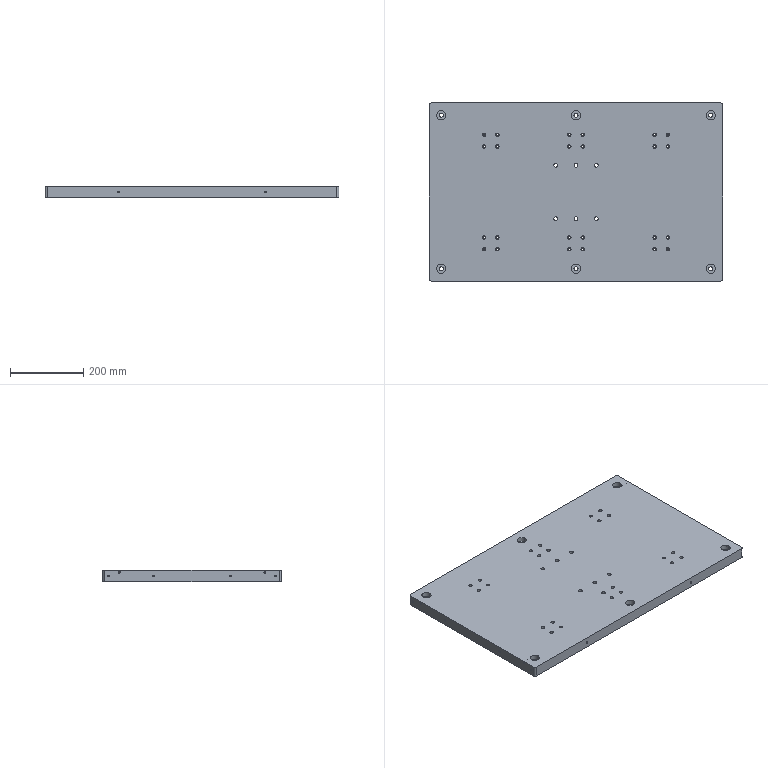NC program | Mastercam | posted with a generic post | part box 800 x 485 x 30 mm
Lines 761 to 1452 of 3510:
( X+CL )
N7560 T20 M6
N7570 G0 G90 G17 G54 X-261.1 Y118. A0. S4000 M3
N7580 G43 H20 Z50. M8
N7590 Z1.2
N7600 G1 Z.2 F600.
N7610 X-259.1 F3000.
N7620 G3 X-257.1 Y120. I0. J2.
N7630 X-265. Y127.9 Z-.05 I-7.9 J0.
N7640 X-272.9 Y120. Z-.3 I0. J-7.9
N7650 X-265. Y112.1 Z-.55 I7.9 J0.
N7660 X-257.1 Y120. Z-.8 I0. J7.9
N7670 X-265. Y127.9 Z-1.05 I-7.9 J0.
N7680 X-272.9 Y120. Z-1.3 I0. J-7.9
N7690 X-265. Y112.1 Z-1.55 I7.9 J0.
N7700 X-257.1 Y120. Z-1.8 I0. J7.9
N7710 X-265. Y127.9 Z-2.05 I-7.9 J0.
N7720 X-272.9 Y120. Z-2.3 I0. J-7.9
N7730 X-265. Y112.1 Z-2.55 I7.9 J0.
N7740 X-257.1 Y120. Z-2.8 I0. J7.9
N7750 X-265. Y127.9 Z-3.05 I-7.9 J0.
N7760 X-272.9 Y120. Z-3.3 I0. J-7.9
N7770 X-265. Y112.1 Z-3.55 I7.9 J0.
N7780 X-257.1 Y120. Z-3.8 I0. J7.9
N7790 X-265. Y127.9 Z-4.05 I-7.9 J0.
N7800 X-272.9 Y120. Z-4.3 I0. J-7.9
N7810 X-265. Y112.1 Z-4.55 I7.9 J0.
N7820 X-257.1 Y120. Z-4.8 I0. J7.9
N7830 X-265. Y127.9 Z-5.05 I-7.9 J0.
N7840 X-272.9 Y120. Z-5.3 I0. J-7.9
N7850 X-265. Y112.1 Z-5.55 I7.9 J0.
N7860 X-257.1 Y120. Z-5.8 I0. J7.9
N7870 X-265. Y127.9 Z-6.05 I-7.9 J0.
N7880 X-272.9 Y120. Z-6.3 I0. J-7.9
N7890 X-265. Y112.1 Z-6.55 I7.9 J0.
N7900 X-257.1 Y120. Z-6.8 I0. J7.9
N7910 X-265. Y127.9 Z-7.05 I-7.9 J0.
N7920 X-272.9 Y120. Z-7.3 I0. J-7.9
N7930 X-265. Y112.1 Z-7.55 I7.9 J0.
N7940 X-257.1 Y120. Z-7.8 I0. J7.9
N7950 X-265. Y127.9 Z-8.05 I-7.9 J0.
N7960 X-272.9 Y120. Z-8.3 I0. J-7.9
N7970 X-265. Y112.1 Z-8.55 I7.9 J0.
N7980 X-257.1 Y120. Z-8.8 I0. J7.9
N7990 X-265. Y127.9 Z-9.05 I-7.9 J0.
N8000 X-272.9 Y120. Z-9.3 I0. J-7.9
N8010 X-265. Y112.1 Z-9.55 I7.9 J0.
N8020 X-257.1 Y120. Z-9.8 I0. J7.9
N8030 X-265. Y127.9 Z-10.05 I-7.9 J0.
N8040 X-272.9 Y120. Z-10.3 I0. J-7.9
N8050 X-265. Y112.1 Z-10.55 I7.9 J0.
N8060 X-257.1 Y120. Z-10.8 I0. J7.9
N8070 X-265. Y127.9 Z-11.05 I-7.9 J0.
N8080 X-272.9 Y120. Z-11.3 I0. J-7.9
N8090 X-265. Y112.1 Z-11.55 I7.9 J0.
N8100 X-257.1 Y120. Z-11.8 I0. J7.9
N8110 X-265. Y127.9 Z-12.05 I-7.9 J0.
N8120 X-272.9 Y120. Z-12.3 I0. J-7.9
N8130 X-265. Y112.1 Z-12.55 I7.9 J0.
N8140 X-257.1 Y120. Z-12.8 I0. J7.9
N8150 X-265. Y127.9 Z-13.05 I-7.9 J0.
N8160 X-272.9 Y120. Z-13.3 I0. J-7.9
N8170 X-265. Y112.1 Z-13.55 I7.9 J0.
N8180 X-257.1 Y120. Z-13.8 I0. J7.9
N8190 X-265. Y127.9 Z-14.05 I-7.9 J0.
N8200 X-272.9 Y120. Z-14.3 I0. J-7.9
N8210 X-265. Y112.1 Z-14.55 I7.9 J0.
N8220 X-257.1 Y120. Z-14.8 I0. J7.9
N8230 X-265. Y127.9 Z-15.05 I-7.9 J0.
N8240 X-272.9 Y120. Z-15.3 I0. J-7.9
N8250 X-265. Y112.1 Z-15.55 I7.9 J0.
N8260 X-257.1 Y120. Z-15.8 I0. J7.9
N8270 X-265. Y127.9 Z-16.05 I-7.9 J0.
N8280 X-272.9 Y120. Z-16.3 I0. J-7.9
N8290 X-265. Y112.1 Z-16.55 I7.9 J0.
N8300 X-257.1 Y120. Z-16.8 I0. J7.9
N8310 X-265. Y127.9 Z-17.05 I-7.9 J0.
N8320 X-272.9 Y120. Z-17.3 I0. J-7.9
N8330 X-265. Y112.1 Z-17.55 I7.9 J0.
N8340 X-257.1 Y120. Z-17.8 I0. J7.9
N8350 X-265. Y127.9 Z-18.05 I-7.9 J0.
N8360 X-272.9 Y120. Z-18.3 I0. J-7.9
N8370 X-265. Y112.1 Z-18.55 I7.9 J0.
N8380 X-257.1 Y120. Z-18.8 I0. J7.9
N8390 X-265. Y127.9 Z-19.05 I-7.9 J0.
N8400 X-272.9 Y120. Z-19.3 I0. J-7.9
N8410 X-265. Y112.1 Z-19.55 I7.9 J0.
N8420 X-257.1 Y120. Z-19.8 I0. J7.9
N8430 X-265. Y127.9 Z-20.05 I-7.9 J0.
N8440 X-272.9 Y120. Z-20.3 I0. J-7.9
N8450 X-265. Y112.1 Z-20.55 I7.9 J0.
N8460 X-257.1 Y120. Z-20.8 I0. J7.9
N8470 X-265. Y127.9 Z-21.05 I-7.9 J0.
N8480 X-272.9 Y120. Z-21.3 I0. J-7.9
N8490 X-265. Y112.1 Z-21.55 I7.9 J0.
N8500 X-257.1 Y120. Z-21.8 I0. J7.9
N8510 X-265. Y127.9 Z-22.05 I-7.9 J0.
N8520 X-272.9 Y120. Z-22.3 I0. J-7.9
N8530 X-265. Y112.1 Z-22.55 I7.9 J0.
N8540 X-257.1 Y120. Z-22.8 I0. J7.9
N8550 X-265. Y127.9 Z-23.05 I-7.9 J0.
N8560 X-272.9 Y120. Z-23.3 I0. J-7.9
N8570 X-265. Y112.1 Z-23.55 I7.9 J0.
N8580 X-257.1 Y120. Z-23.8 I0. J7.9
N8590 X-265. Y127.9 Z-24.05 I-7.9 J0.
N8600 X-272.9 Y120. Z-24.3 I0. J-7.9
N8610 X-265. Y112.1 Z-24.55 I7.9 J0.
N8620 X-257.1 Y120. Z-24.8 I0. J7.9
N8630 X-260.356 Y126.391 Z-24.95 I-7.9 J0.
N8640 X-265. Y127.9 I-4.644 J-6.391
N8650 X-272.9 Y120. I0. J-7.9
N8660 X-265. Y112.1 I7.9 J0.
N8670 X-257.1 Y120. I0. J7.9
N8680 X-260.356 Y126.391 I-7.9 J0.
N8690 X-261.532 Y126.773 I-1.176 J-1.618
N8700 X-263.15 Y125.949 I0. J-2.
N8710 G1 X-264.326 Y124.331
N8720 G0 Z50.
N8730 X-251.1 Y118.
N8740 Z1.2
N8750 G1 Z.2 F600.
N8760 X-249.1 F3000.
N8770 G3 X-247.1 Y120. I0. J2.
N8780 X-265. Y137.9 Z-.05 I-17.9 J0.
N8790 X-282.9 Y120. Z-.3 I0. J-17.9
N8800 X-265. Y102.1 Z-.55 I17.9 J0.
N8810 X-247.1 Y120. Z-.8 I0. J17.9
N8820 X-265. Y137.9 Z-1.05 I-17.9 J0.
N8830 X-282.9 Y120. Z-1.3 I0. J-17.9
N8840 X-265. Y102.1 Z-1.55 I17.9 J0.
N8850 X-247.1 Y120. Z-1.8 I0. J17.9
N8860 X-265. Y137.9 Z-2.05 I-17.9 J0.
N8870 X-282.9 Y120. Z-2.3 I0. J-17.9
N8880 X-265. Y102.1 Z-2.55 I17.9 J0.
N8890 X-247.1 Y120. Z-2.8 I0. J17.9
N8900 X-265. Y137.9 Z-3.05 I-17.9 J0.
N8910 X-282.9 Y120. Z-3.3 I0. J-17.9
N8920 X-265. Y102.1 Z-3.55 I17.9 J0.
N8930 X-247.1 Y120. Z-3.8 I0. J17.9
N8940 X-265. Y137.9 Z-4.05 I-17.9 J0.
N8950 X-282.9 Y120. Z-4.3 I0. J-17.9
N8960 X-265. Y102.1 Z-4.55 I17.9 J0.
N8970 X-247.1 Y120. Z-4.8 I0. J17.9
N8980 X-265. Y137.9 Z-5.05 I-17.9 J0.
N8990 X-282.9 Y120. Z-5.3 I0. J-17.9
N9000 X-265. Y102.1 Z-5.55 I17.9 J0.
N9010 X-247.1 Y120. Z-5.8 I0. J17.9
N9020 X-265. Y137.9 Z-6.05 I-17.9 J0.
N9030 X-282.9 Y120. Z-6.3 I0. J-17.9
N9040 X-265. Y102.1 Z-6.55 I17.9 J0.
N9050 X-247.1 Y120. Z-6.8 I0. J17.9
N9060 X-265. Y137.9 Z-7.05 I-17.9 J0.
N9070 X-282.9 Y120. Z-7.3 I0. J-17.9
N9080 X-265. Y102.1 Z-7.55 I17.9 J0.
N9090 X-247.1 Y120. Z-7.8 I0. J17.9
N9100 X-265. Y137.9 Z-8.05 I-17.9 J0.
N9110 X-282.9 Y120. Z-8.3 I0. J-17.9
N9120 X-265. Y102.1 Z-8.55 I17.9 J0.
N9130 X-247.1 Y120. Z-8.8 I0. J17.9
N9140 X-265. Y137.9 Z-9.05 I-17.9 J0.
N9150 X-282.9 Y120. Z-9.3 I0. J-17.9
N9160 X-265. Y102.1 Z-9.55 I17.9 J0.
N9170 X-247.1 Y120. Z-9.8 I0. J17.9
N9180 X-265. Y137.9 Z-10.05 I-17.9 J0.
N9190 X-282.9 Y120. Z-10.3 I0. J-17.9
N9200 X-265. Y102.1 Z-10.55 I17.9 J0.
N9210 X-247.1 Y120. Z-10.8 I0. J17.9
N9220 X-265. Y137.9 Z-11.05 I-17.9 J0.
N9230 X-282.9 Y120. Z-11.3 I0. J-17.9
N9240 X-265. Y102.1 Z-11.55 I17.9 J0.
N9250 X-247.1 Y120. Z-11.8 I0. J17.9
N9260 X-265. Y137.9 Z-12.05 I-17.9 J0.
N9270 X-282.9 Y120. Z-12.3 I0. J-17.9
N9280 X-265. Y102.1 Z-12.55 I17.9 J0.
N9290 X-247.1 Y120. Z-12.8 I0. J17.9
N9300 X-265. Y137.9 Z-13.05 I-17.9 J0.
N9310 X-282.9 Y120. Z-13.3 I0. J-17.9
N9320 X-265. Y102.1 Z-13.55 I17.9 J0.
N9330 X-247.1 Y120. Z-13.8 I0. J17.9
N9340 X-265. Y137.9 Z-14.05 I-17.9 J0.
N9350 X-282.9 Y120. Z-14.3 I0. J-17.9
N9360 X-265. Y102.1 Z-14.55 I17.9 J0.
N9370 X-247.1 Y120. Z-14.8 I0. J17.9
N9380 X-265. Y137.9 Z-15.05 I-17.9 J0.
N9390 X-282.9 Y120. Z-15.3 I0. J-17.9
N9400 X-265. Y102.1 Z-15.55 I17.9 J0.
N9410 X-247.1 Y120. Z-15.8 I0. J17.9
N9420 X-265. Y137.9 Z-16.05 I-17.9 J0.
N9430 X-282.9 Y120. Z-16.3 I0. J-17.9
N9440 X-265. Y102.1 Z-16.55 I17.9 J0.
N9450 X-247.1 Y120. Z-16.8 I0. J17.9
N9460 X-265. Y137.9 Z-17.05 I-17.9 J0.
N9470 X-282.9 Y120. Z-17.3 I0. J-17.9
N9480 X-265. Y102.1 Z-17.55 I17.9 J0.
N9490 X-247.1 Y120. Z-17.8 I0. J17.9
N9500 X-265. Y137.9 Z-18.05 I-17.9 J0.
N9510 X-282.9 Y120. Z-18.3 I0. J-17.9
N9520 X-265. Y102.1 Z-18.55 I17.9 J0.
N9530 X-247.1 Y120. Z-18.8 I0. J17.9
N9540 X-265. Y137.9 Z-19.05 I-17.9 J0.
N9550 X-282.9 Y120. Z-19.3 I0. J-17.9
N9560 X-265. Y102.1 Z-19.55 I17.9 J0.
N9570 X-247.1 Y120. Z-19.8 I0. J17.9
N9580 X-265. Y137.9 Z-20.05 I-17.9 J0.
N9590 X-282.9 Y120. Z-20.3 I0. J-17.9
N9600 X-265. Y102.1 Z-20.55 I17.9 J0.
N9610 X-247.1 Y120. Z-20.8 I0. J17.9
N9620 X-265. Y137.9 Z-21.05 I-17.9 J0.
N9630 X-282.9 Y120. Z-21.3 I0. J-17.9
N9640 X-265. Y102.1 Z-21.55 I17.9 J0.
N9650 X-247.1 Y120. Z-21.8 I0. J17.9
N9660 X-265. Y137.9 Z-22.05 I-17.9 J0.
N9670 X-282.9 Y120. Z-22.3 I0. J-17.9
N9680 X-265. Y102.1 Z-22.55 I17.9 J0.
N9690 X-247.1 Y120. Z-22.8 I0. J17.9
N9700 X-265. Y137.9 Z-23.05 I-17.9 J0.
N9710 X-282.9 Y120. Z-23.3 I0. J-17.9
N9720 X-265. Y102.1 Z-23.55 I17.9 J0.
N9730 X-247.1 Y120. Z-23.8 I0. J17.9
N9740 X-265. Y137.9 Z-24.05 I-17.9 J0.
N9750 X-282.9 Y120. Z-24.3 I0. J-17.9
N9760 X-265. Y102.1 Z-24.55 I17.9 J0.
N9770 X-247.1 Y120. Z-24.8 I0. J17.9
N9780 X-254.479 Y134.481 Z-24.95 I-17.9 J0.
N9790 X-265. Y137.899 I-10.521 J-14.481
N9800 X-282.899 Y120. I0. J-17.899
N9810 X-265. Y102.101 I17.899 J0.
N9820 X-247.1 Y120. I0. J17.899
N9830 X-254.479 Y134.481 I-17.9 J0.
N9840 X-255.654 Y134.863 I-1.175 J-1.618
N9850 X-257.272 Y134.039 I0. J-2.
N9860 G1 X-258.448 Y132.421
N9870 G0 Z50.
N9880 X3.9 Y118.
N9890 Z1.2
N9900 G1 Z.2 F600.
N9910 X5.9 F3000.
N9920 G3 X7.9 Y120. I0. J2.
N9930 X0. Y127.9 Z-.05 I-7.9 J0.
N9940 X-7.9 Y120. Z-.3 I0. J-7.9
N9950 X0. Y112.1 Z-.55 I7.9 J0.
N9960 X7.9 Y120. Z-.8 I0. J7.9
N9970 X0. Y127.9 Z-1.05 I-7.9 J0.
N9980 X-7.9 Y120. Z-1.3 I0. J-7.9
N9990 X0. Y112.1 Z-1.55 I7.9 J0.
N100 X7.9 Y120. Z-1.8 I0. J7.9
N110 X0. Y127.9 Z-2.05 I-7.9 J0.
N120 X-7.9 Y120. Z-2.3 I0. J-7.9
N130 X0. Y112.1 Z-2.55 I7.9 J0.
N140 X7.9 Y120. Z-2.8 I0. J7.9
N150 X0. Y127.9 Z-3.05 I-7.9 J0.
N160 X-7.9 Y120. Z-3.3 I0. J-7.9
N170 X0. Y112.1 Z-3.55 I7.9 J0.
N180 X7.9 Y120. Z-3.8 I0. J7.9
N190 X0. Y127.9 Z-4.05 I-7.9 J0.
N200 X-7.9 Y120. Z-4.3 I0. J-7.9
N210 X0. Y112.1 Z-4.55 I7.9 J0.
N220 X7.9 Y120. Z-4.8 I0. J7.9
N230 X0. Y127.9 Z-5.05 I-7.9 J0.
N240 X-7.9 Y120. Z-5.3 I0. J-7.9
N250 X0. Y112.1 Z-5.55 I7.9 J0.
N260 X7.9 Y120. Z-5.8 I0. J7.9
N270 X0. Y127.9 Z-6.05 I-7.9 J0.
N280 X-7.9 Y120. Z-6.3 I0. J-7.9
N290 X0. Y112.1 Z-6.55 I7.9 J0.
N300 X7.9 Y120. Z-6.8 I0. J7.9
N310 X0. Y127.9 Z-7.05 I-7.9 J0.
N320 X-7.9 Y120. Z-7.3 I0. J-7.9
N330 X0. Y112.1 Z-7.55 I7.9 J0.
N340 X7.9 Y120. Z-7.8 I0. J7.9
N350 X0. Y127.9 Z-8.05 I-7.9 J0.
N360 X-7.9 Y120. Z-8.3 I0. J-7.9
N370 X0. Y112.1 Z-8.55 I7.9 J0.
N380 X7.9 Y120. Z-8.8 I0. J7.9
N390 X0. Y127.9 Z-9.05 I-7.9 J0.
N400 X-7.9 Y120. Z-9.3 I0. J-7.9
N410 X0. Y112.1 Z-9.55 I7.9 J0.
N420 X7.9 Y120. Z-9.8 I0. J7.9
N430 X0. Y127.9 Z-10.05 I-7.9 J0.
N440 X-7.9 Y120. Z-10.3 I0. J-7.9
N450 X0. Y112.1 Z-10.55 I7.9 J0.
N460 X7.9 Y120. Z-10.8 I0. J7.9
N470 X0. Y127.9 Z-11.05 I-7.9 J0.
N480 X-7.9 Y120. Z-11.3 I0. J-7.9
N490 X0. Y112.1 Z-11.55 I7.9 J0.
N500 X7.9 Y120. Z-11.8 I0. J7.9
N510 X0. Y127.9 Z-12.05 I-7.9 J0.
N520 X-7.9 Y120. Z-12.3 I0. J-7.9
N530 X0. Y112.1 Z-12.55 I7.9 J0.
N540 X7.9 Y120. Z-12.8 I0. J7.9
N550 X0. Y127.9 Z-13.05 I-7.9 J0.
N560 X-7.9 Y120. Z-13.3 I0. J-7.9
N570 X0. Y112.1 Z-13.55 I7.9 J0.
N580 X7.9 Y120. Z-13.8 I0. J7.9
N590 X0. Y127.9 Z-14.05 I-7.9 J0.
N600 X-7.9 Y120. Z-14.3 I0. J-7.9
N610 X0. Y112.1 Z-14.55 I7.9 J0.
N620 X7.9 Y120. Z-14.8 I0. J7.9
N630 X0. Y127.9 Z-15.05 I-7.9 J0.
N640 X-7.9 Y120. Z-15.3 I0. J-7.9
N650 X0. Y112.1 Z-15.55 I7.9 J0.
N660 X7.9 Y120. Z-15.8 I0. J7.9
N670 X0. Y127.9 Z-16.05 I-7.9 J0.
N680 X-7.9 Y120. Z-16.3 I0. J-7.9
N690 X0. Y112.1 Z-16.55 I7.9 J0.
N700 X7.9 Y120. Z-16.8 I0. J7.9
N710 X0. Y127.9 Z-17.05 I-7.9 J0.
N720 X-7.9 Y120. Z-17.3 I0. J-7.9
N730 X0. Y112.1 Z-17.55 I7.9 J0.
N740 X7.9 Y120. Z-17.8 I0. J7.9
N750 X0. Y127.9 Z-18.05 I-7.9 J0.
N760 X-7.9 Y120. Z-18.3 I0. J-7.9
N770 X0. Y112.1 Z-18.55 I7.9 J0.
N780 X7.9 Y120. Z-18.8 I0. J7.9
N790 X0. Y127.9 Z-19.05 I-7.9 J0.
N800 X-7.9 Y120. Z-19.3 I0. J-7.9
N810 X0. Y112.1 Z-19.55 I7.9 J0.
N820 X7.9 Y120. Z-19.8 I0. J7.9
N830 X0. Y127.9 Z-20.05 I-7.9 J0.
N840 X-7.9 Y120. Z-20.3 I0. J-7.9
N850 X0. Y112.1 Z-20.55 I7.9 J0.
N860 X7.9 Y120. Z-20.8 I0. J7.9
N870 X0. Y127.9 Z-21.05 I-7.9 J0.
N880 X-7.9 Y120. Z-21.3 I0. J-7.9
N890 X0. Y112.1 Z-21.55 I7.9 J0.
N900 X7.9 Y120. Z-21.8 I0. J7.9
N910 X0. Y127.9 Z-22.05 I-7.9 J0.
N920 X-7.9 Y120. Z-22.3 I0. J-7.9
N930 X0. Y112.1 Z-22.55 I7.9 J0.
N940 X7.9 Y120. Z-22.8 I0. J7.9
N950 X0. Y127.9 Z-23.05 I-7.9 J0.
N960 X-7.9 Y120. Z-23.3 I0. J-7.9
N970 X0. Y112.1 Z-23.55 I7.9 J0.
N980 X7.9 Y120. Z-23.8 I0. J7.9
N990 X0. Y127.9 Z-24.05 I-7.9 J0.
N1000 X-7.9 Y120. Z-24.3 I0. J-7.9
N1010 X0. Y112.1 Z-24.55 I7.9 J0.
N1020 X7.9 Y120. Z-24.8 I0. J7.9
N1030 X4.644 Y126.391 Z-24.95 I-7.9 J0.
N1040 X0. Y127.9 I-4.644 J-6.391
N1050 X-7.9 Y120. I0. J-7.9
N1060 X0. Y112.1 I7.9 J0.
N1070 X7.9 Y120. I0. J7.9
N1080 X4.644 Y126.391 I-7.9 J0.
N1090 X3.468 Y126.773 I-1.176 J-1.618
N1100 X1.85 Y125.949 I0. J-2.
N1110 G1 X.674 Y124.331
N1120 G0 Z50.
N1130 X13.9 Y118.
N1140 Z1.2
N1150 G1 Z.2 F600.
N1160 X15.9 F3000.
N1170 G3 X17.9 Y120. I0. J2.
N1180 X0. Y137.9 Z-.05 I-17.9 J0.
N1190 X-17.9 Y120. Z-.3 I0. J-17.9
N1200 X0. Y102.1 Z-.55 I17.9 J0.
N1210 X17.9 Y120. Z-.8 I0. J17.9
N1220 X0. Y137.9 Z-1.05 I-17.9 J0.
N1230 X-17.9 Y120. Z-1.3 I0. J-17.9
N1240 X0. Y102.1 Z-1.55 I17.9 J0.
N1250 X17.9 Y120. Z-1.8 I0. J17.9
N1260 X0. Y137.9 Z-2.05 I-17.9 J0.
N1270 X-17.9 Y120. Z-2.3 I0. J-17.9
N1280 X0. Y102.1 Z-2.55 I17.9 J0.
N1290 X17.9 Y120. Z-2.8 I0. J17.9
N1300 X0. Y137.9 Z-3.05 I-17.9 J0.
N1310 X-17.9 Y120. Z-3.3 I0. J-17.9
N1320 X0. Y102.1 Z-3.55 I17.9 J0.
N1330 X17.9 Y120. Z-3.8 I0. J17.9
N1340 X0. Y137.9 Z-4.05 I-17.9 J0.
N1350 X-17.9 Y120. Z-4.3 I0. J-17.9
N1360 X0. Y102.1 Z-4.55 I17.9 J0.
N1370 X17.9 Y120. Z-4.8 I0. J17.9
N1380 X0. Y137.9 Z-5.05 I-17.9 J0.
N1390 X-17.9 Y120. Z-5.3 I0. J-17.9
N1400 X0. Y102.1 Z-5.55 I17.9 J0.
N1410 X17.9 Y120. Z-5.8 I0. J17.9
N1420 X0. Y137.9 Z-6.05 I-17.9 J0.
N1430 X-17.9 Y120. Z-6.3 I0. J-17.9
N1440 X0. Y102.1 Z-6.55 I17.9 J0.
N1450 X17.9 Y120. Z-6.8 I0. J17.9
N1460 X0. Y137.9 Z-7.05 I-17.9 J0.
N1470 X-17.9 Y120. Z-7.3 I0. J-17.9
N1480 X0. Y102.1 Z-7.55 I17.9 J0.
N1490 X17.9 Y120. Z-7.8 I0. J17.9
N1500 X0. Y137.9 Z-8.05 I-17.9 J0.
N1510 X-17.9 Y120. Z-8.3 I0. J-17.9
N1520 X0. Y102.1 Z-8.55 I17.9 J0.
N1530 X17.9 Y120. Z-8.8 I0. J17.9
N1540 X0. Y137.9 Z-9.05 I-17.9 J0.
N1550 X-17.9 Y120. Z-9.3 I0. J-17.9
N1560 X0. Y102.1 Z-9.55 I17.9 J0.
N1570 X17.9 Y120. Z-9.8 I0. J17.9
N1580 X0. Y137.9 Z-10.05 I-17.9 J0.
N1590 X-17.9 Y120. Z-10.3 I0. J-17.9
N1600 X0. Y102.1 Z-10.55 I17.9 J0.
N1610 X17.9 Y120. Z-10.8 I0. J17.9
N1620 X0. Y137.9 Z-11.05 I-17.9 J0.
N1630 X-17.9 Y120. Z-11.3 I0. J-17.9
N1640 X0. Y102.1 Z-11.55 I17.9 J0.
N1650 X17.9 Y120. Z-11.8 I0. J17.9
N1660 X0. Y137.9 Z-12.05 I-17.9 J0.
N1670 X-17.9 Y120. Z-12.3 I0. J-17.9
N1680 X0. Y102.1 Z-12.55 I17.9 J0.
N1690 X17.9 Y120. Z-12.8 I0. J17.9
N1700 X0. Y137.9 Z-13.05 I-17.9 J0.
N1710 X-17.9 Y120. Z-13.3 I0. J-17.9
N1720 X0. Y102.1 Z-13.55 I17.9 J0.
N1730 X17.9 Y120. Z-13.8 I0. J17.9
N1740 X0. Y137.9 Z-14.05 I-17.9 J0.
N1750 X-17.9 Y120. Z-14.3 I0. J-17.9
N1760 X0. Y102.1 Z-14.55 I17.9 J0.
N1770 X17.9 Y120. Z-14.8 I0. J17.9
N1780 X0. Y137.9 Z-15.05 I-17.9 J0.
N1790 X-17.9 Y120. Z-15.3 I0. J-17.9
N1800 X0. Y102.1 Z-15.55 I17.9 J0.
N1810 X17.9 Y120. Z-15.8 I0. J17.9
N1820 X0. Y137.9 Z-16.05 I-17.9 J0.
N1830 X-17.9 Y120. Z-16.3 I0. J-17.9
N1840 X0. Y102.1 Z-16.55 I17.9 J0.
N1850 X17.9 Y120. Z-16.8 I0. J17.9
N1860 X0. Y137.9 Z-17.05 I-17.9 J0.
N1870 X-17.9 Y120. Z-17.3 I0. J-17.9
N1880 X0. Y102.1 Z-17.55 I17.9 J0.
N1890 X17.9 Y120. Z-17.8 I0. J17.9
N1900 X0. Y137.9 Z-18.05 I-17.9 J0.
N1910 X-17.9 Y120. Z-18.3 I0. J-17.9
N1920 X0. Y102.1 Z-18.55 I17.9 J0.
N1930 X17.9 Y120. Z-18.8 I0. J17.9
N1940 X0. Y137.9 Z-19.05 I-17.9 J0.
N1950 X-17.9 Y120. Z-19.3 I0. J-17.9
N1960 X0. Y102.1 Z-19.55 I17.9 J0.
N1970 X17.9 Y120. Z-19.8 I0. J17.9
N1980 X0. Y137.9 Z-20.05 I-17.9 J0.
N1990 X-17.9 Y120. Z-20.3 I0. J-17.9
N2000 X0. Y102.1 Z-20.55 I17.9 J0.
N2010 X17.9 Y120. Z-20.8 I0. J17.9
N2020 X0. Y137.9 Z-21.05 I-17.9 J0.
N2030 X-17.9 Y120. Z-21.3 I0. J-17.9
N2040 X0. Y102.1 Z-21.55 I17.9 J0.
N2050 X17.9 Y120. Z-21.8 I0. J17.9
N2060 X0. Y137.9 Z-22.05 I-17.9 J0.
N2070 X-17.9 Y120. Z-22.3 I0. J-17.9
N2080 X0. Y102.1 Z-22.55 I17.9 J0.
N2090 X17.9 Y120. Z-22.8 I0. J17.9
N2100 X0. Y137.9 Z-23.05 I-17.9 J0.
N2110 X-17.9 Y120. Z-23.3 I0. J-17.9
N2120 X0. Y102.1 Z-23.55 I17.9 J0.
N2130 X17.9 Y120. Z-23.8 I0. J17.9
N2140 X0. Y137.9 Z-24.05 I-17.9 J0.
N2150 X-17.9 Y120. Z-24.3 I0. J-17.9
N2160 X0. Y102.1 Z-24.55 I17.9 J0.
N2170 X17.9 Y120. Z-24.8 I0. J17.9
N2180 X10.521 Y134.481 Z-24.95 I-17.9 J0.
N2190 X0. Y137.899 I-10.521 J-14.481
N2200 X-17.899 Y120. I0. J-17.899
N2210 X0. Y102.101 I17.899 J0.
N2220 X17.9 Y120. I0. J17.899
N2230 X10.521 Y134.481 I-17.9 J0.
N2240 X9.346 Y134.863 I-1.175 J-1.618
N2250 X7.728 Y134.039 I0. J-2.
N2260 G1 X6.552 Y132.421
N2270 G0 Z50.
N2280 X268.9 Y118.
N2290 Z1.2
N2300 G1 Z.2 F600.
N2310 X270.9 F3000.
N2320 G3 X272.9 Y120. I0. J2.
N2330 X265. Y127.9 Z-.05 I-7.9 J0.
N2340 X257.1 Y120. Z-.3 I0. J-7.9
N2350 X265. Y112.1 Z-.55 I7.9 J0.
N2360 X272.9 Y120. Z-.8 I0. J7.9
N2370 X265. Y127.9 Z-1.05 I-7.9 J0.
N2380 X257.1 Y120. Z-1.3 I0. J-7.9
N2390 X265. Y112.1 Z-1.55 I7.9 J0.
N2400 X272.9 Y120. Z-1.8 I0. J7.9
N2410 X265. Y127.9 Z-2.05 I-7.9 J0.
N2420 X257.1 Y120. Z-2.3 I0. J-7.9
N2430 X265. Y112.1 Z-2.55 I7.9 J0.
N2440 X272.9 Y120. Z-2.8 I0. J7.9
N2450 X265. Y127.9 Z-3.05 I-7.9 J0.
N2460 X257.1 Y120. Z-3.3 I0. J-7.9
N2470 X265. Y112.1 Z-3.55 I7.9 J0.
N2480 X272.9 Y120. Z-3.8 I0. J7.9
N2490 X265. Y127.9 Z-4.05 I-7.9 J0.
N2500 X257.1 Y120. Z-4.3 I0. J-7.9
N2510 X265. Y112.1 Z-4.55 I7.9 J0.
N2520 X272.9 Y120. Z-4.8 I0. J7.9
N2530 X265. Y127.9 Z-5.05 I-7.9 J0.
N2540 X257.1 Y120. Z-5.3 I0. J-7.9
N2550 X265. Y112.1 Z-5.55 I7.9 J0.
N2560 X272.9 Y120. Z-5.8 I0. J7.9
N2570 X265. Y127.9 Z-6.05 I-7.9 J0.
N2580 X257.1 Y120. Z-6.3 I0. J-7.9
N2590 X265. Y112.1 Z-6.55 I7.9 J0.
N2600 X272.9 Y120. Z-6.8 I0. J7.9
N2610 X265. Y127.9 Z-7.05 I-7.9 J0.
N2620 X257.1 Y120. Z-7.3 I0. J-7.9
N2630 X265. Y112.1 Z-7.55 I7.9 J0.
N2640 X272.9 Y120. Z-7.8 I0. J7.9
N2650 X265. Y127.9 Z-8.05 I-7.9 J0.
N2660 X257.1 Y120. Z-8.3 I0. J-7.9
N2670 X265. Y112.1 Z-8.55 I7.9 J0.
N2680 X272.9 Y120. Z-8.8 I0. J7.9
N2690 X265. Y127.9 Z-9.05 I-7.9 J0.
N2700 X257.1 Y120. Z-9.3 I0. J-7.9
N2710 X265. Y112.1 Z-9.55 I7.9 J0.
N2720 X272.9 Y120. Z-9.8 I0. J7.9
N2730 X265. Y127.9 Z-10.05 I-7.9 J0.
N2740 X257.1 Y120. Z-10.3 I0. J-7.9
N2750 X265. Y112.1 Z-10.55 I7.9 J0.
N2760 X272.9 Y120. Z-10.8 I0. J7.9
N2770 X265. Y127.9 Z-11.05 I-7.9 J0.
N2780 X257.1 Y120. Z-11.3 I0. J-7.9
N2790 X265. Y112.1 Z-11.55 I7.9 J0.
N2800 X272.9 Y120. Z-11.8 I0. J7.9
N2810 X265. Y127.9 Z-12.05 I-7.9 J0.
N2820 X257.1 Y120. Z-12.3 I0. J-7.9
N2830 X265. Y112.1 Z-12.55 I7.9 J0.
N2840 X272.9 Y120. Z-12.8 I0. J7.9
N2850 X265. Y127.9 Z-13.05 I-7.9 J0.
N2860 X257.1 Y120. Z-13.3 I0. J-7.9
N2870 X265. Y112.1 Z-13.55 I7.9 J0.
N2880 X272.9 Y120. Z-13.8 I0. J7.9
N2890 X265. Y127.9 Z-14.05 I-7.9 J0.
N2900 X257.1 Y120. Z-14.3 I0. J-7.9
N2910 X265. Y112.1 Z-14.55 I7.9 J0.
N2920 X272.9 Y120. Z-14.8 I0. J7.9
N2930 X265. Y127.9 Z-15.05 I-7.9 J0.
N2940 X257.1 Y120. Z-15.3 I0. J-7.9
N2950 X265. Y112.1 Z-15.55 I7.9 J0.
N2960 X272.9 Y120. Z-15.8 I0. J7.9
N2970 X265. Y127.9 Z-16.05 I-7.9 J0.
N2980 X257.1 Y120. Z-16.3 I0. J-7.9
N2990 X265. Y112.1 Z-16.55 I7.9 J0.
N3000 X272.9 Y120. Z-16.8 I0. J7.9
N3010 X265. Y127.9 Z-17.05 I-7.9 J0.
N3020 X257.1 Y120. Z-17.3 I0. J-7.9
N3030 X265. Y112.1 Z-17.55 I7.9 J0.
N3040 X272.9 Y120. Z-17.8 I0. J7.9
N3050 X265. Y127.9 Z-18.05 I-7.9 J0.
N3060 X257.1 Y120. Z-18.3 I0. J-7.9
N3070 X265. Y112.1 Z-18.55 I7.9 J0.
N3080 X272.9 Y120. Z-18.8 I0. J7.9
N3090 X265. Y127.9 Z-19.05 I-7.9 J0.
N3100 X257.1 Y120. Z-19.3 I0. J-7.9
N3110 X265. Y112.1 Z-19.55 I7.9 J0.
N3120 X272.9 Y120. Z-19.8 I0. J7.9
N3130 X265. Y127.9 Z-20.05 I-7.9 J0.
N3140 X257.1 Y120. Z-20.3 I0. J-7.9
N3150 X265. Y112.1 Z-20.55 I7.9 J0.
N3160 X272.9 Y120. Z-20.8 I0. J7.9
N3170 X265. Y127.9 Z-21.05 I-7.9 J0.
N3180 X257.1 Y120. Z-21.3 I0. J-7.9
N3190 X265. Y112.1 Z-21.55 I7.9 J0.
N3200 X272.9 Y120. Z-21.8 I0. J7.9
N3210 X265. Y127.9 Z-22.05 I-7.9 J0.
N3220 X257.1 Y120. Z-22.3 I0. J-7.9
N3230 X265. Y112.1 Z-22.55 I7.9 J0.
N3240 X272.9 Y120. Z-22.8 I0. J7.9
N3250 X265. Y127.9 Z-23.05 I-7.9 J0.
N3260 X257.1 Y120. Z-23.3 I0. J-7.9
N3270 X265. Y112.1 Z-23.55 I7.9 J0.
N3280 X272.9 Y120. Z-23.8 I0. J7.9
N3290 X265. Y127.9 Z-24.05 I-7.9 J0.
N3300 X257.1 Y120. Z-24.3 I0. J-7.9
N3310 X265. Y112.1 Z-24.55 I7.9 J0.
N3320 X272.9 Y120. Z-24.8 I0. J7.9
N3330 X269.644 Y126.391 Z-24.95 I-7.9 J0.
N3340 X265. Y127.9 I-4.644 J-6.391
N3350 X257.1 Y120. I0. J-7.9
N3360 X265. Y112.1 I7.9 J0.
N3370 X272.9 Y120. I0. J7.9
N3380 X269.644 Y126.391 I-7.9 J0.
N3390 X268.468 Y126.773 I-1.176 J-1.618
N3400 X266.85 Y125.949 I0. J-2.
N3410 G1 X265.674 Y124.331
N3420 G0 Z50.
N3430 X278.9 Y118.
N3440 Z1.2
N3450 G1 Z.2 F600.
N3460 X280.9 F3000.
N3470 G3 X282.9 Y120. I0. J2.
N3480 X265. Y137.9 Z-.05 I-17.9 J0.
N3490 X247.1 Y120. Z-.3 I0. J-17.9
N3500 X265. Y102.1 Z-.55 I17.9 J0.
N3510 X282.9 Y120. Z-.8 I0. J17.9
N3520 X265. Y137.9 Z-1.05 I-17.9 J0.
N3530 X247.1 Y120. Z-1.3 I0. J-17.9
N3540 X265. Y102.1 Z-1.55 I17.9 J0.
N3550 X282.9 Y120. Z-1.8 I0. J17.9
N3560 X265. Y137.9 Z-2.05 I-17.9 J0.
N3570 X247.1 Y120. Z-2.3 I0. J-17.9
N3580 X265. Y102.1 Z-2.55 I17.9 J0.
N3590 X282.9 Y120. Z-2.8 I0. J17.9
N3600 X265. Y137.9 Z-3.05 I-17.9 J0.
N3610 X247.1 Y120. Z-3.3 I0. J-17.9
N3620 X265. Y102.1 Z-3.55 I17.9 J0.
N3630 X282.9 Y120. Z-3.8 I0. J17.9
N3640 X265. Y137.9 Z-4.05 I-17.9 J0.
N3650 X247.1 Y120. Z-4.3 I0. J-17.9
N3660 X265. Y102.1 Z-4.55 I17.9 J0.
N3670 X282.9 Y120. Z-4.8 I0. J17.9
N3680 X265. Y137.9 Z-5.05 I-17.9 J0.
N3690 X247.1 Y120. Z-5.3 I0. J-17.9
N3700 X265. Y102.1 Z-5.55 I17.9 J0.
N3710 X282.9 Y120. Z-5.8 I0. J17.9
N3720 X265. Y137.9 Z-6.05 I-17.9 J0.
N3730 X247.1 Y120. Z-6.3 I0. J-17.9
N3740 X265. Y102.1 Z-6.55 I17.9 J0.
N3750 X282.9 Y120. Z-6.8 I0. J17.9
N3760 X265. Y137.9 Z-7.05 I-17.9 J0.
N3770 X247.1 Y120. Z-7.3 I0. J-17.9
N3780 X265. Y102.1 Z-7.55 I17.9 J0.
N3790 X282.9 Y120. Z-7.8 I0. J17.9
N3800 X265. Y137.9 Z-8.05 I-17.9 J0.
N3810 X247.1 Y120. Z-8.3 I0. J-17.9
N3820 X265. Y102.1 Z-8.55 I17.9 J0.
N3830 X282.9 Y120. Z-8.8 I0. J17.9
N3840 X265. Y137.9 Z-9.05 I-17.9 J0.
N3850 X247.1 Y120. Z-9.3 I0. J-17.9
N3860 X265. Y102.1 Z-9.55 I17.9 J0.
N3870 X282.9 Y120. Z-9.8 I0. J17.9
N3880 X265. Y137.9 Z-10.05 I-17.9 J0.
N3890 X247.1 Y120. Z-10.3 I0. J-17.9
N3900 X265. Y102.1 Z-10.55 I17.9 J0.
N3910 X282.9 Y120. Z-10.8 I0. J17.9
N3920 X265. Y137.9 Z-11.05 I-17.9 J0.
N3930 X247.1 Y120. Z-11.3 I0. J-17.9
N3940 X265. Y102.1 Z-11.55 I17.9 J0.
N3950 X282.9 Y120. Z-11.8 I0. J17.9
N3960 X265. Y137.9 Z-12.05 I-17.9 J0.
N3970 X247.1 Y120. Z-12.3 I0. J-17.9
N3980 X265. Y102.1 Z-12.55 I17.9 J0.
N3990 X282.9 Y120. Z-12.8 I0. J17.9
N4000 X265. Y137.9 Z-13.05 I-17.9 J0.
N4010 X247.1 Y120. Z-13.3 I0. J-17.9
N4020 X265. Y102.1 Z-13.55 I17.9 J0.
N4030 X282.9 Y120. Z-13.8 I0. J17.9
N4040 X265. Y137.9 Z-14.05 I-17.9 J0.
N4050 X247.1 Y120. Z-14.3 I0. J-17.9
N4060 X265. Y102.1 Z-14.55 I17.9 J0.
N4070 X282.9 Y120. Z-14.8 I0. J17.9
N4080 X265. Y137.9 Z-15.05 I-17.9 J0.
N4090 X247.1 Y120. Z-15.3 I0. J-17.9
N4100 X265. Y102.1 Z-15.55 I17.9 J0.
N4110 X282.9 Y120. Z-15.8 I0. J17.9
N4120 X265. Y137.9 Z-16.05 I-17.9 J0.
N4130 X247.1 Y120. Z-16.3 I0. J-17.9
N4140 X265. Y102.1 Z-16.55 I17.9 J0.
N4150 X282.9 Y120. Z-16.8 I0. J17.9
N4160 X265. Y137.9 Z-17.05 I-17.9 J0.
N4170 X247.1 Y120. Z-17.3 I0. J-17.9
N4180 X265. Y102.1 Z-17.55 I17.9 J0.
N4190 X282.9 Y120. Z-17.8 I0. J17.9
N4200 X265. Y137.9 Z-18.05 I-17.9 J0.
N4210 X247.1 Y120. Z-18.3 I0. J-17.9
N4220 X265. Y102.1 Z-18.55 I17.9 J0.
N4230 X282.9 Y120. Z-18.8 I0. J17.9
N4240 X265. Y137.9 Z-19.05 I-17.9 J0.
N4250 X247.1 Y120. Z-19.3 I0. J-17.9
N4260 X265. Y102.1 Z-19.55 I17.9 J0.
N4270 X282.9 Y120. Z-19.8 I0. J17.9
N4280 X265. Y137.9 Z-20.05 I-17.9 J0.
N4290 X247.1 Y120. Z-20.3 I0. J-17.9
N4300 X265. Y102.1 Z-20.55 I17.9 J0.
N4310 X282.9 Y120. Z-20.8 I0. J17.9
N4320 X265. Y137.9 Z-21.05 I-17.9 J0.
N4330 X247.1 Y120. Z-21.3 I0. J-17.9
N4340 X265. Y102.1 Z-21.55 I17.9 J0.
N4350 X282.9 Y120. Z-21.8 I0. J17.9
N4360 X265. Y137.9 Z-22.05 I-17.9 J0.
N4370 X247.1 Y120. Z-22.3 I0. J-17.9
N4380 X265. Y102.1 Z-22.55 I17.9 J0.
N4390 X282.9 Y120. Z-22.8 I0. J17.9
N4400 X265. Y137.9 Z-23.05 I-17.9 J0.
N4410 X247.1 Y120. Z-23.3 I0. J-17.9
N4420 X265. Y102.1 Z-23.55 I17.9 J0.
N4430 X282.9 Y120. Z-23.8 I0. J17.9
N4440 X265. Y137.9 Z-24.05 I-17.9 J0.
N4450 X247.1 Y120. Z-24.3 I0. J-17.9
N4460 X265. Y102.1 Z-24.55 I17.9 J0.
N4470 X282.9 Y120. Z-24.8 I0. J17.9
N4480 X275.521 Y134.481 Z-24.95 I-17.9 J0.
N4490 X265. Y137.899 I-10.521 J-14.481
N4500 X247.101 Y120. I0. J-17.899
N4510 X265. Y102.101 I17.899 J0.
N4520 X282.9 Y120. I0. J17.899
N4530 X275.521 Y134.481 I-17.9 J0.
N4540 X274.346 Y134.863 I-1.175 J-1.618
N4550 X272.728 Y134.039 I0. J-2.
N4560 G1 X271.552 Y132.421